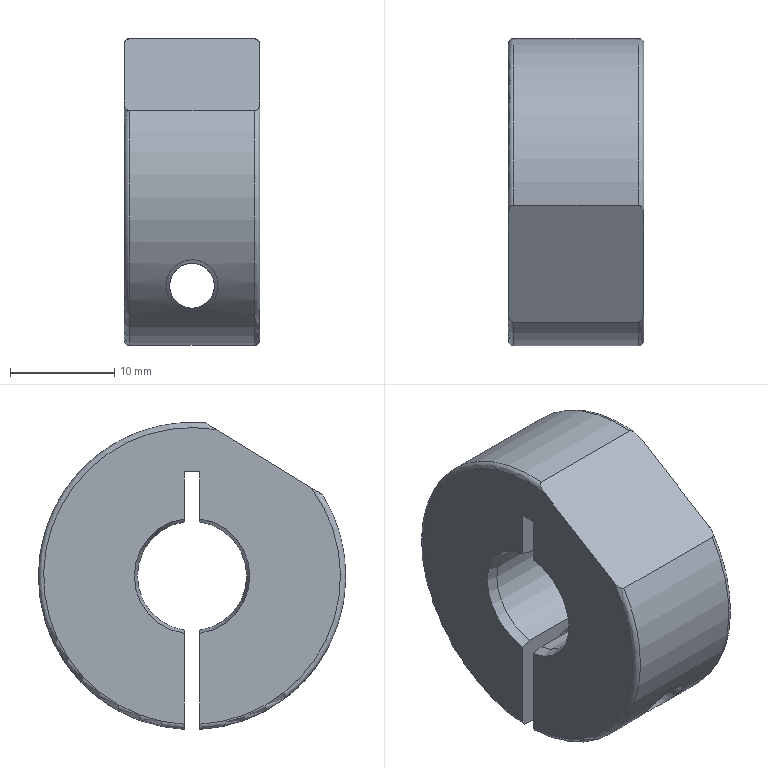Part | STEP file | P0503100005_D | 1 solid | 25 faces | box 13 x 29.5 x 29.481 mm | volume 6728 mm3 | plane 9 | cylinder 8 | torus 4 | cone 4 | commonest cylinder face diameters 10.5 x2 29.5 x2 4.3 x1 5 x1 5.6 x1 9.5 x1